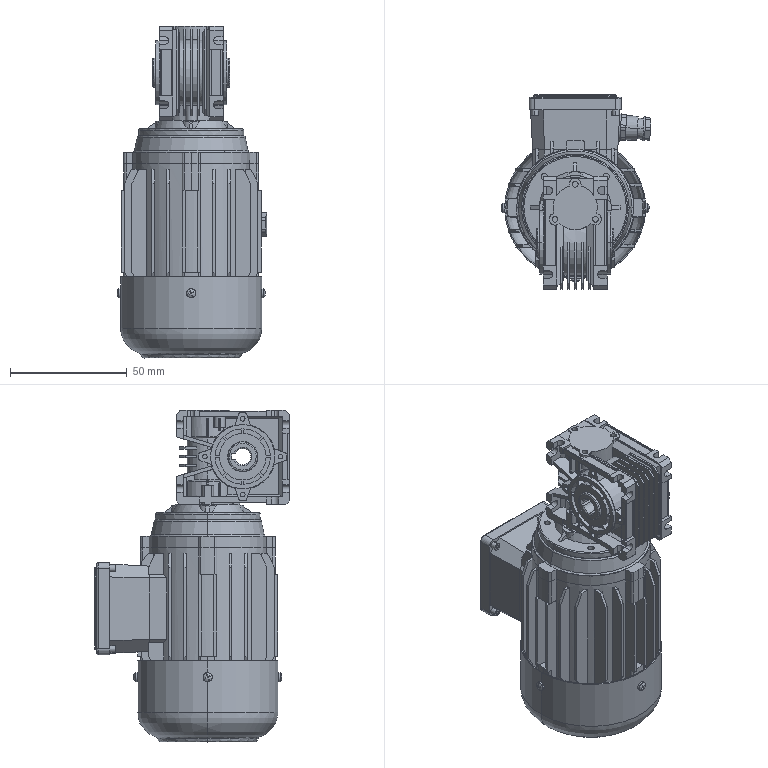Part | SolidWorks | features BaseBody 11, Scale 1 | 11 solids | 1787 faces | box 64.261 x 83.502 x 142.348 mm | volume 222279 mm3 | plane 922 | cylinder 564 | spline 199 | cone 98 | torus 4 | commonest cylinder face diameters 1 x116 0.5 x65 2 x46 3 x34 5 x29 2.5 x25